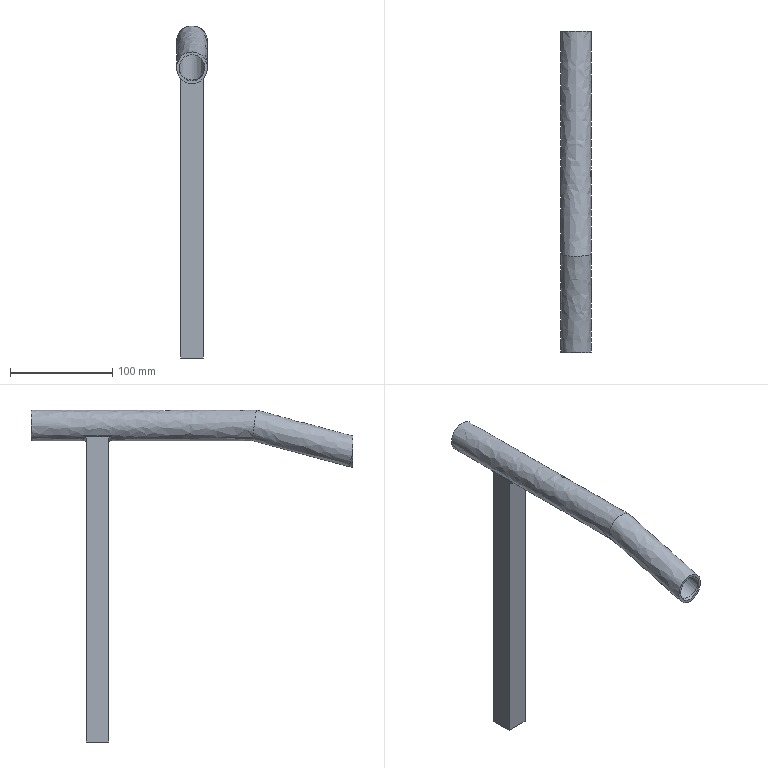Part | NX | features solid 2 | 1 solid | 22 faces | box 30 x 315.001 x 325 mm | volume 127017 mm3 | plane 11 | spline 10 | cylinder 1 | commonest cylinder face diameters 30 x1